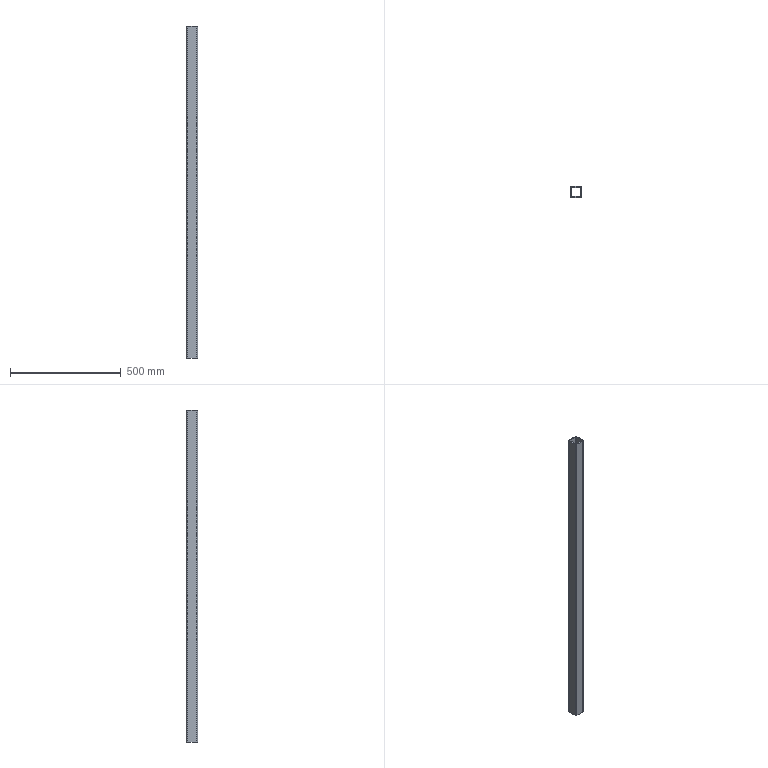Part | SolidWorks | features Extrusion 1 | 1 solid | 18 faces | box 50 x 50 x 1500 mm | volume 1304934 mm3 | plane 10 | cylinder 8 | commonest cylinder face diameters 2 x4 12 x4
STEP:
#1=CARTESIAN_POINT('',(0.,6.,1500.));
#2=VERTEX_POINT('',#1);
#3=CARTESIAN_POINT('',(6.,0.,1500.));
#4=VERTEX_POINT('',#3);
#5=CARTESIAN_POINT('',(6.,6.,1500.));
#6=DIRECTION('',(0.,0.,1.));
#7=DIRECTION('',(-1.,0.,0.));
#8=AXIS2_PLACEMENT_3D('',#5,#6,#7);
#9=CIRCLE('',#8,6.);
#10=EDGE_CURVE('',#2,#4,#9,.T.);
#11=ORIENTED_EDGE('',*,*,#10,.T.);
#12=CARTESIAN_POINT('',(44.,0.,1500.));
#13=VERTEX_POINT('',#12);
#14=CARTESIAN_POINT('',(6.,0.,1500.));
#15=DIRECTION('',(1.,0.,0.));
#16=VECTOR('',#15,1000.);
#17=LINE('',#14,#16);
#18=EDGE_CURVE('',#4,#13,#17,.T.);
#19=ORIENTED_EDGE('',*,*,#18,.T.);
#20=CARTESIAN_POINT('',(50.,6.,1500.));
#21=VERTEX_POINT('',#20);
#22=CARTESIAN_POINT('',(44.,6.,1500.));
#23=DIRECTION('',(0.,0.,1.));
#24=DIRECTION('',(1.,0.,0.));
#25=AXIS2_PLACEMENT_3D('',#22,#23,#24);
#26=CIRCLE('',#25,6.);
#27=EDGE_CURVE('',#13,#21,#26,.T.);
#28=ORIENTED_EDGE('',*,*,#27,.T.);
#29=CARTESIAN_POINT('',(50.,44.,1500.));
#30=VERTEX_POINT('',#29);
#31=CARTESIAN_POINT('',(50.,6.,1500.));
#32=DIRECTION('',(0.,1.,0.));
#33=VECTOR('',#32,1000.);
#34=LINE('',#31,#33);
#35=EDGE_CURVE('',#21,#30,#34,.T.);
#36=ORIENTED_EDGE('',*,*,#35,.T.);
#37=CARTESIAN_POINT('',(44.,50.,1500.));
#38=VERTEX_POINT('',#37);
#39=CARTESIAN_POINT('',(44.,44.,1500.));
#40=DIRECTION('',(0.,0.,1.));
#41=DIRECTION('',(-1.,0.,0.));
#42=AXIS2_PLACEMENT_3D('',#39,#40,#41);
#43=CIRCLE('',#42,6.);
#44=EDGE_CURVE('',#30,#38,#43,.T.);
#45=ORIENTED_EDGE('',*,*,#44,.T.);
#46=CARTESIAN_POINT('',(6.,50.,1500.));
#47=VERTEX_POINT('',#46);
#48=CARTESIAN_POINT('',(6.,50.,1500.));
#49=DIRECTION('',(-1.,0.,0.));
#50=VECTOR('',#49,1000.);
#51=LINE('',#48,#50);
#52=EDGE_CURVE('',#38,#47,#51,.T.);
#53=ORIENTED_EDGE('',*,*,#52,.T.);
#54=CARTESIAN_POINT('',(0.,44.,1500.));
#55=VERTEX_POINT('',#54);
#56=CARTESIAN_POINT('',(6.,44.,1500.));
#57=DIRECTION('',(0.,0.,1.));
#58=DIRECTION('',(-1.,0.,0.));
#59=AXIS2_PLACEMENT_3D('',#56,#57,#58);
#60=CIRCLE('',#59,6.);
#61=EDGE_CURVE('',#47,#55,#60,.T.);
#62=ORIENTED_EDGE('',*,*,#61,.T.);
#63=CARTESIAN_POINT('',(0.,6.,1500.));
#64=DIRECTION('',(0.,-1.,0.));
#65=VECTOR('',#64,1000.);
#66=LINE('',#63,#65);
#67=EDGE_CURVE('',#55,#2,#66,.T.);
#68=ORIENTED_EDGE('',*,*,#67,.T.);
#69=EDGE_LOOP('',(#11,#19,#28,#36,#45,#53,#62,#68));
#70=FACE_OUTER_BOUND('',#69,.T.);
#71=CARTESIAN_POINT('',(6.,45.,1500.));
#72=VERTEX_POINT('',#71);
#73=CARTESIAN_POINT('',(5.,44.,1500.));
#74=VERTEX_POINT('',#73);
#75=CARTESIAN_POINT('',(6.,44.,1500.));
#76=DIRECTION('',(0.,0.,1.));
#77=DIRECTION('',(-1.,0.,0.));
#78=AXIS2_PLACEMENT_3D('',#75,#76,#77);
#79=CIRCLE('',#78,1.);
#80=EDGE_CURVE('',#72,#74,#79,.T.);
#81=ORIENTED_EDGE('',*,*,#80,.F.);
#82=CARTESIAN_POINT('',(44.,45.,1500.));
#83=VERTEX_POINT('',#82);
#84=CARTESIAN_POINT('',(6.,45.,1500.));
#85=DIRECTION('',(-1.,0.,0.));
#86=VECTOR('',#85,1000.);
#87=LINE('',#84,#86);
#88=EDGE_CURVE('',#83,#72,#87,.T.);
#89=ORIENTED_EDGE('',*,*,#88,.F.);
#90=CARTESIAN_POINT('',(45.,44.,1500.));
#91=VERTEX_POINT('',#90);
#92=CARTESIAN_POINT('',(44.,44.,1500.));
#93=DIRECTION('',(0.,0.,1.));
#94=DIRECTION('',(-1.,0.,0.));
#95=AXIS2_PLACEMENT_3D('',#92,#93,#94);
#96=CIRCLE('',#95,1.);
#97=EDGE_CURVE('',#91,#83,#96,.T.);
#98=ORIENTED_EDGE('',*,*,#97,.F.);
#99=CARTESIAN_POINT('',(45.,6.,1500.));
#100=VERTEX_POINT('',#99);
#101=CARTESIAN_POINT('',(45.,6.,1500.));
#102=DIRECTION('',(0.,1.,0.));
#103=VECTOR('',#102,1000.);
#104=LINE('',#101,#103);
#105=EDGE_CURVE('',#100,#91,#104,.T.);
#106=ORIENTED_EDGE('',*,*,#105,.F.);
#107=CARTESIAN_POINT('',(44.,5.,1500.));
#108=VERTEX_POINT('',#107);
#109=CARTESIAN_POINT('',(44.,6.,1500.));
#110=DIRECTION('',(0.,0.,1.));
#111=DIRECTION('',(1.,0.,0.));
#112=AXIS2_PLACEMENT_3D('',#109,#110,#111);
#113=CIRCLE('',#112,1.);
#114=EDGE_CURVE('',#108,#100,#113,.T.);
#115=ORIENTED_EDGE('',*,*,#114,.F.);
#116=CARTESIAN_POINT('',(6.,5.,1500.));
#117=VERTEX_POINT('',#116);
#118=CARTESIAN_POINT('',(6.,5.,1500.));
#119=DIRECTION('',(1.,0.,0.));
#120=VECTOR('',#119,1000.);
#121=LINE('',#118,#120);
#122=EDGE_CURVE('',#117,#108,#121,.T.);
#123=ORIENTED_EDGE('',*,*,#122,.F.);
#124=CARTESIAN_POINT('',(5.,6.,1500.));
#125=VERTEX_POINT('',#124);
#126=CARTESIAN_POINT('',(6.,6.,1500.));
#127=DIRECTION('',(0.,0.,1.));
#128=DIRECTION('',(-1.,0.,0.));
#129=AXIS2_PLACEMENT_3D('',#126,#127,#128);
#130=CIRCLE('',#129,1.);
#131=EDGE_CURVE('',#125,#117,#130,.T.);
#132=ORIENTED_EDGE('',*,*,#131,.F.);
#133=CARTESIAN_POINT('',(5.,6.,1500.));
#134=DIRECTION('',(0.,-1.,0.));
#135=VECTOR('',#134,1000.);
#136=LINE('',#133,#135);
#137=EDGE_CURVE('',#74,#125,#136,.T.);
#138=ORIENTED_EDGE('',*,*,#137,.F.);
#139=EDGE_LOOP('',(#81,#89,#98,#106,#115,#123,#132,#138));
#140=FACE_BOUND('',#139,.T.);
#141=CARTESIAN_POINT('',(6.,6.,1500.));
#142=DIRECTION('',(0.,0.,-1.));
#143=DIRECTION('',(-1.,0.,0.));
#144=AXIS2_PLACEMENT_3D('',#141,#142,#143);
#145=PLANE('',#144);
#146=ADVANCED_FACE('',(#70,#140),#145,.F.);
#147=CARTESIAN_POINT('',(0.,6.,0.));
#148=VERTEX_POINT('',#147);
#149=CARTESIAN_POINT('',(6.,0.,0.));
#150=VERTEX_POINT('',#149);
#151=CARTESIAN_POINT('',(6.,6.,0.));
#152=DIRECTION('',(0.,0.,1.));
#153=DIRECTION('',(-1.,0.,0.));
#154=AXIS2_PLACEMENT_3D('',#151,#152,#153);
#155=CIRCLE('',#154,6.);
#156=EDGE_CURVE('',#148,#150,#155,.T.);
#157=ORIENTED_EDGE('',*,*,#156,.F.);
#158=CARTESIAN_POINT('',(0.,44.,0.));
#159=VERTEX_POINT('',#158);
#160=CARTESIAN_POINT('',(0.,6.,0.));
#161=DIRECTION('',(0.,-1.,0.));
#162=VECTOR('',#161,1000.);
#163=LINE('',#160,#162);
#164=EDGE_CURVE('',#159,#148,#163,.T.);
#165=ORIENTED_EDGE('',*,*,#164,.F.);
#166=CARTESIAN_POINT('',(6.,50.,0.));
#167=VERTEX_POINT('',#166);
#168=CARTESIAN_POINT('',(6.,44.,0.));
#169=DIRECTION('',(0.,0.,1.));
#170=DIRECTION('',(-1.,0.,0.));
#171=AXIS2_PLACEMENT_3D('',#168,#169,#170);
#172=CIRCLE('',#171,6.);
#173=EDGE_CURVE('',#167,#159,#172,.T.);
#174=ORIENTED_EDGE('',*,*,#173,.F.);
#175=CARTESIAN_POINT('',(44.,50.,0.));
#176=VERTEX_POINT('',#175);
#177=CARTESIAN_POINT('',(6.,50.,0.));
#178=DIRECTION('',(-1.,0.,0.));
#179=VECTOR('',#178,1000.);
#180=LINE('',#177,#179);
#181=EDGE_CURVE('',#176,#167,#180,.T.);
#182=ORIENTED_EDGE('',*,*,#181,.F.);
#183=CARTESIAN_POINT('',(50.,44.,0.));
#184=VERTEX_POINT('',#183);
#185=CARTESIAN_POINT('',(44.,44.,0.));
#186=DIRECTION('',(0.,0.,1.));
#187=DIRECTION('',(-1.,0.,0.));
#188=AXIS2_PLACEMENT_3D('',#185,#186,#187);
#189=CIRCLE('',#188,6.);
#190=EDGE_CURVE('',#184,#176,#189,.T.);
#191=ORIENTED_EDGE('',*,*,#190,.F.);
#192=CARTESIAN_POINT('',(50.,6.,0.));
#193=VERTEX_POINT('',#192);
#194=CARTESIAN_POINT('',(50.,6.,0.));
#195=DIRECTION('',(0.,1.,0.));
#196=VECTOR('',#195,1000.);
#197=LINE('',#194,#196);
#198=EDGE_CURVE('',#193,#184,#197,.T.);
#199=ORIENTED_EDGE('',*,*,#198,.F.);
#200=CARTESIAN_POINT('',(44.,0.,0.));
#201=VERTEX_POINT('',#200);
#202=CARTESIAN_POINT('',(44.,6.,0.));
#203=DIRECTION('',(0.,0.,1.));
#204=DIRECTION('',(1.,0.,0.));
#205=AXIS2_PLACEMENT_3D('',#202,#203,#204);
#206=CIRCLE('',#205,6.);
#207=EDGE_CURVE('',#201,#193,#206,.T.);
#208=ORIENTED_EDGE('',*,*,#207,.F.);
#209=CARTESIAN_POINT('',(6.,0.,0.));
#210=DIRECTION('',(1.,0.,0.));
#211=VECTOR('',#210,1000.);
#212=LINE('',#209,#211);
#213=EDGE_CURVE('',#150,#201,#212,.T.);
#214=ORIENTED_EDGE('',*,*,#213,.F.);
#215=EDGE_LOOP('',(#157,#165,#174,#182,#191,#199,#208,#214));
#216=FACE_OUTER_BOUND('',#215,.T.);
#217=CARTESIAN_POINT('',(44.,45.,0.));
#218=VERTEX_POINT('',#217);
#219=CARTESIAN_POINT('',(6.,45.,0.));
#220=VERTEX_POINT('',#219);
#221=CARTESIAN_POINT('',(6.,45.,0.));
#222=DIRECTION('',(-1.,0.,0.));
#223=VECTOR('',#222,1000.);
#224=LINE('',#221,#223);
#225=EDGE_CURVE('',#218,#220,#224,.T.);
#226=ORIENTED_EDGE('',*,*,#225,.T.);
#227=CARTESIAN_POINT('',(5.,44.,0.));
#228=VERTEX_POINT('',#227);
#229=CARTESIAN_POINT('',(6.,44.,0.));
#230=DIRECTION('',(0.,0.,1.));
#231=DIRECTION('',(-1.,0.,0.));
#232=AXIS2_PLACEMENT_3D('',#229,#230,#231);
#233=CIRCLE('',#232,1.);
#234=EDGE_CURVE('',#220,#228,#233,.T.);
#235=ORIENTED_EDGE('',*,*,#234,.T.);
#236=CARTESIAN_POINT('',(5.,6.,0.));
#237=VERTEX_POINT('',#236);
#238=CARTESIAN_POINT('',(5.,6.,0.));
#239=DIRECTION('',(0.,-1.,0.));
#240=VECTOR('',#239,1000.);
#241=LINE('',#238,#240);
#242=EDGE_CURVE('',#228,#237,#241,.T.);
#243=ORIENTED_EDGE('',*,*,#242,.T.);
#244=CARTESIAN_POINT('',(6.,5.,0.));
#245=VERTEX_POINT('',#244);
#246=CARTESIAN_POINT('',(6.,6.,0.));
#247=DIRECTION('',(0.,0.,1.));
#248=DIRECTION('',(-1.,0.,0.));
#249=AXIS2_PLACEMENT_3D('',#246,#247,#248);
#250=CIRCLE('',#249,1.);
#251=EDGE_CURVE('',#237,#245,#250,.T.);
#252=ORIENTED_EDGE('',*,*,#251,.T.);
#253=CARTESIAN_POINT('',(44.,5.,0.));
#254=VERTEX_POINT('',#253);
#255=CARTESIAN_POINT('',(6.,5.,0.));
#256=DIRECTION('',(1.,0.,0.));
#257=VECTOR('',#256,1000.);
#258=LINE('',#255,#257);
#259=EDGE_CURVE('',#245,#254,#258,.T.);
#260=ORIENTED_EDGE('',*,*,#259,.T.);
#261=CARTESIAN_POINT('',(45.,6.,0.));
#262=VERTEX_POINT('',#261);
#263=CARTESIAN_POINT('',(44.,6.,0.));
#264=DIRECTION('',(0.,0.,1.));
#265=DIRECTION('',(1.,0.,0.));
#266=AXIS2_PLACEMENT_3D('',#263,#264,#265);
#267=CIRCLE('',#266,1.);
#268=EDGE_CURVE('',#254,#262,#267,.T.);
#269=ORIENTED_EDGE('',*,*,#268,.T.);
#270=CARTESIAN_POINT('',(45.,44.,0.));
#271=VERTEX_POINT('',#270);
#272=CARTESIAN_POINT('',(45.,6.,0.));
#273=DIRECTION('',(0.,1.,0.));
#274=VECTOR('',#273,1000.);
#275=LINE('',#272,#274);
#276=EDGE_CURVE('',#262,#271,#275,.T.);
#277=ORIENTED_EDGE('',*,*,#276,.T.);
#278=CARTESIAN_POINT('',(44.,44.,0.));
#279=DIRECTION('',(0.,0.,1.));
#280=DIRECTION('',(-1.,0.,0.));
#281=AXIS2_PLACEMENT_3D('',#278,#279,#280);
#282=CIRCLE('',#281,1.);
#283=EDGE_CURVE('',#271,#218,#282,.T.);
#284=ORIENTED_EDGE('',*,*,#283,.T.);
#285=EDGE_LOOP('',(#226,#235,#243,#252,#260,#269,#277,#284));
#286=FACE_BOUND('',#285,.T.);
#287=CARTESIAN_POINT('',(6.,6.,0.));
#288=DIRECTION('',(0.,0.,-1.));
#289=DIRECTION('',(-1.,0.,0.));
#290=AXIS2_PLACEMENT_3D('',#287,#288,#289);
#291=PLANE('',#290);
#292=ADVANCED_FACE('',(#216,#286),#291,.T.);
#293=ORIENTED_EDGE('',*,*,#156,.T.);
#294=CARTESIAN_POINT('',(6.,0.,1500.));
#295=DIRECTION('',(0.,0.,-1.));
#296=VECTOR('',#295,1000.);
#297=LINE('',#294,#296);
#298=EDGE_CURVE('',#4,#150,#297,.T.);
#299=ORIENTED_EDGE('',*,*,#298,.F.);
#300=ORIENTED_EDGE('',*,*,#10,.F.);
#301=CARTESIAN_POINT('',(0.,6.,1500.));
#302=DIRECTION('',(0.,0.,-1.));
#303=VECTOR('',#302,1000.);
#304=LINE('',#301,#303);
#305=EDGE_CURVE('',#2,#148,#304,.T.);
#306=ORIENTED_EDGE('',*,*,#305,.T.);
#307=EDGE_LOOP('',(#293,#299,#300,#306));
#308=FACE_OUTER_BOUND('',#307,.T.);
#309=CARTESIAN_POINT('',(6.,6.,1500.));
#310=DIRECTION('',(0.,0.,-1.));
#311=DIRECTION('',(-1.,0.,0.));
#312=AXIS2_PLACEMENT_3D('',#309,#310,#311);
#313=CYLINDRICAL_SURFACE('',#312,6.);
#314=ADVANCED_FACE('',(#308),#313,.T.);
#315=ORIENTED_EDGE('',*,*,#213,.T.);
#316=CARTESIAN_POINT('',(44.,0.,1500.));
#317=DIRECTION('',(0.,0.,-1.));
#318=VECTOR('',#317,1000.);
#319=LINE('',#316,#318);
#320=EDGE_CURVE('',#13,#201,#319,.T.);
#321=ORIENTED_EDGE('',*,*,#320,.F.);
#322=ORIENTED_EDGE('',*,*,#18,.F.);
#323=ORIENTED_EDGE('',*,*,#298,.T.);
#324=EDGE_LOOP('',(#315,#321,#322,#323));
#325=FACE_OUTER_BOUND('',#324,.T.);
#326=CARTESIAN_POINT('',(6.,0.,1500.));
#327=DIRECTION('',(0.,1.,0.));
#328=DIRECTION('',(0.,0.,1.));
#329=AXIS2_PLACEMENT_3D('',#326,#327,#328);
#330=PLANE('',#329);
#331=ADVANCED_FACE('',(#325),#330,.F.);
#332=ORIENTED_EDGE('',*,*,#207,.T.);
#333=CARTESIAN_POINT('',(50.,6.,1500.));
#334=DIRECTION('',(0.,0.,-1.));
#335=VECTOR('',#334,1000.);
#336=LINE('',#333,#335);
#337=EDGE_CURVE('',#21,#193,#336,.T.);
#338=ORIENTED_EDGE('',*,*,#337,.F.);
#339=ORIENTED_EDGE('',*,*,#27,.F.);
#340=ORIENTED_EDGE('',*,*,#320,.T.);
#341=EDGE_LOOP('',(#332,#338,#339,#340));
#342=FACE_OUTER_BOUND('',#341,.T.);
#343=CARTESIAN_POINT('',(44.,6.,1500.));
#344=DIRECTION('',(0.,0.,-1.));
#345=DIRECTION('',(-1.,0.,0.));
#346=AXIS2_PLACEMENT_3D('',#343,#344,#345);
#347=CYLINDRICAL_SURFACE('',#346,6.);
#348=ADVANCED_FACE('',(#342),#347,.T.);
#349=ORIENTED_EDGE('',*,*,#198,.T.);
#350=CARTESIAN_POINT('',(50.,44.,1500.));
#351=DIRECTION('',(0.,0.,-1.));
#352=VECTOR('',#351,1000.);
#353=LINE('',#350,#352);
#354=EDGE_CURVE('',#30,#184,#353,.T.);
#355=ORIENTED_EDGE('',*,*,#354,.F.);
#356=ORIENTED_EDGE('',*,*,#35,.F.);
#357=ORIENTED_EDGE('',*,*,#337,.T.);
#358=EDGE_LOOP('',(#349,#355,#356,#357));
#359=FACE_OUTER_BOUND('',#358,.T.);
#360=CARTESIAN_POINT('',(50.,6.,1500.));
#361=DIRECTION('',(-1.,0.,0.));
#362=DIRECTION('',(0.,0.,1.));
#363=AXIS2_PLACEMENT_3D('',#360,#361,#362);
#364=PLANE('',#363);
#365=ADVANCED_FACE('',(#359),#364,.F.);
#366=ORIENTED_EDGE('',*,*,#190,.T.);
#367=CARTESIAN_POINT('',(44.,50.,1500.));
#368=DIRECTION('',(0.,0.,-1.));
#369=VECTOR('',#368,1000.);
#370=LINE('',#367,#369);
#371=EDGE_CURVE('',#38,#176,#370,.T.);
#372=ORIENTED_EDGE('',*,*,#371,.F.);
#373=ORIENTED_EDGE('',*,*,#44,.F.);
#374=ORIENTED_EDGE('',*,*,#354,.T.);
#375=EDGE_LOOP('',(#366,#372,#373,#374));
#376=FACE_OUTER_BOUND('',#375,.T.);
#377=CARTESIAN_POINT('',(44.,44.,1500.));
#378=DIRECTION('',(0.,0.,-1.));
#379=DIRECTION('',(-1.,0.,0.));
#380=AXIS2_PLACEMENT_3D('',#377,#378,#379);
#381=CYLINDRICAL_SURFACE('',#380,6.);
#382=ADVANCED_FACE('',(#376),#381,.T.);
#383=ORIENTED_EDGE('',*,*,#181,.T.);
#384=CARTESIAN_POINT('',(6.,50.,1500.));
#385=DIRECTION('',(0.,0.,-1.));
#386=VECTOR('',#385,1000.);
#387=LINE('',#384,#386);
#388=EDGE_CURVE('',#47,#167,#387,.T.);
#389=ORIENTED_EDGE('',*,*,#388,.F.);
#390=ORIENTED_EDGE('',*,*,#52,.F.);
#391=ORIENTED_EDGE('',*,*,#371,.T.);
#392=EDGE_LOOP('',(#383,#389,#390,#391));
#393=FACE_OUTER_BOUND('',#392,.T.);
#394=CARTESIAN_POINT('',(6.,50.,1500.));
#395=DIRECTION('',(0.,-1.,0.));
#396=DIRECTION('',(0.,0.,-1.));
#397=AXIS2_PLACEMENT_3D('',#394,#395,#396);
#398=PLANE('',#397);
#399=ADVANCED_FACE('',(#393),#398,.F.);
#400=ORIENTED_EDGE('',*,*,#173,.T.);
#401=CARTESIAN_POINT('',(0.,44.,1500.));
#402=DIRECTION('',(0.,0.,-1.));
#403=VECTOR('',#402,1000.);
#404=LINE('',#401,#403);
#405=EDGE_CURVE('',#55,#159,#404,.T.);
#406=ORIENTED_EDGE('',*,*,#405,.F.);
#407=ORIENTED_EDGE('',*,*,#61,.F.);
#408=ORIENTED_EDGE('',*,*,#388,.T.);
#409=EDGE_LOOP('',(#400,#406,#407,#408));
#410=FACE_OUTER_BOUND('',#409,.T.);
#411=CARTESIAN_POINT('',(6.,44.,1500.));
#412=DIRECTION('',(0.,0.,-1.));
#413=DIRECTION('',(-1.,0.,0.));
#414=AXIS2_PLACEMENT_3D('',#411,#412,#413);
#415=CYLINDRICAL_SURFACE('',#414,6.);
#416=ADVANCED_FACE('',(#410),#415,.T.);
#417=ORIENTED_EDGE('',*,*,#164,.T.);
#418=ORIENTED_EDGE('',*,*,#305,.F.);
#419=ORIENTED_EDGE('',*,*,#67,.F.);
#420=ORIENTED_EDGE('',*,*,#405,.T.);
#421=EDGE_LOOP('',(#417,#418,#419,#420));
#422=FACE_OUTER_BOUND('',#421,.T.);
#423=CARTESIAN_POINT('',(0.,6.,1500.));
#424=DIRECTION('',(1.,0.,0.));
#425=DIRECTION('',(0.,0.,-1.));
#426=AXIS2_PLACEMENT_3D('',#423,#424,#425);
#427=PLANE('',#426);
#428=ADVANCED_FACE('',(#422),#427,.F.);
#429=ORIENTED_EDGE('',*,*,#234,.F.);
#430=CARTESIAN_POINT('',(6.,45.,1500.));
#431=DIRECTION('',(0.,0.,-1.));
#432=VECTOR('',#431,1000.);
#433=LINE('',#430,#432);
#434=EDGE_CURVE('',#72,#220,#433,.T.);
#435=ORIENTED_EDGE('',*,*,#434,.F.);
#436=ORIENTED_EDGE('',*,*,#80,.T.);
#437=CARTESIAN_POINT('',(5.,44.,1500.));
#438=DIRECTION('',(0.,0.,-1.));
#439=VECTOR('',#438,1000.);
#440=LINE('',#437,#439);
#441=EDGE_CURVE('',#74,#228,#440,.T.);
#442=ORIENTED_EDGE('',*,*,#441,.T.);
#443=EDGE_LOOP('',(#429,#435,#436,#442));
#444=FACE_OUTER_BOUND('',#443,.T.);
#445=CARTESIAN_POINT('',(6.,44.,1500.));
#446=DIRECTION('',(0.,0.,-1.));
#447=DIRECTION('',(-1.,0.,0.));
#448=AXIS2_PLACEMENT_3D('',#445,#446,#447);
#449=CYLINDRICAL_SURFACE('',#448,1.);
#450=ADVANCED_FACE('',(#444),#449,.F.);
#451=ORIENTED_EDGE('',*,*,#242,.F.);
#452=ORIENTED_EDGE('',*,*,#441,.F.);
#453=ORIENTED_EDGE('',*,*,#137,.T.);
#454=CARTESIAN_POINT('',(5.,6.,1500.));
#455=DIRECTION('',(0.,0.,-1.));
#456=VECTOR('',#455,1000.);
#457=LINE('',#454,#456);
#458=EDGE_CURVE('',#125,#237,#457,.T.);
#459=ORIENTED_EDGE('',*,*,#458,.T.);
#460=EDGE_LOOP('',(#451,#452,#453,#459));
#461=FACE_OUTER_BOUND('',#460,.T.);
#462=CARTESIAN_POINT('',(5.,6.,1500.));
#463=DIRECTION('',(1.,0.,0.));
#464=DIRECTION('',(0.,1.,0.));
#465=AXIS2_PLACEMENT_3D('',#462,#463,#464);
#466=PLANE('',#465);
#467=ADVANCED_FACE('',(#461),#466,.T.);
#468=ORIENTED_EDGE('',*,*,#251,.F.);
#469=ORIENTED_EDGE('',*,*,#458,.F.);
#470=ORIENTED_EDGE('',*,*,#131,.T.);
#471=CARTESIAN_POINT('',(6.,5.,1500.));
#472=DIRECTION('',(0.,0.,-1.));
#473=VECTOR('',#472,1000.);
#474=LINE('',#471,#473);
#475=EDGE_CURVE('',#117,#245,#474,.T.);
#476=ORIENTED_EDGE('',*,*,#475,.T.);
#477=EDGE_LOOP('',(#468,#469,#470,#476));
#478=FACE_OUTER_BOUND('',#477,.T.);
#479=CARTESIAN_POINT('',(6.,6.,1500.));
#480=DIRECTION('',(0.,0.,-1.));
#481=DIRECTION('',(-1.,0.,0.));
#482=AXIS2_PLACEMENT_3D('',#479,#480,#481);
#483=CYLINDRICAL_SURFACE('',#482,1.);
#484=ADVANCED_FACE('',(#478),#483,.F.);
#485=ORIENTED_EDGE('',*,*,#259,.F.);
#486=ORIENTED_EDGE('',*,*,#475,.F.);
#487=ORIENTED_EDGE('',*,*,#122,.T.);
#488=CARTESIAN_POINT('',(44.,5.,1500.));
#489=DIRECTION('',(0.,0.,-1.));
#490=VECTOR('',#489,1000.);
#491=LINE('',#488,#490);
#492=EDGE_CURVE('',#108,#254,#491,.T.);
#493=ORIENTED_EDGE('',*,*,#492,.T.);
#494=EDGE_LOOP('',(#485,#486,#487,#493));
#495=FACE_OUTER_BOUND('',#494,.T.);
#496=CARTESIAN_POINT('',(6.,5.,1500.));
#497=DIRECTION('',(0.,1.,0.));
#498=DIRECTION('',(-1.,0.,0.));
#499=AXIS2_PLACEMENT_3D('',#496,#497,#498);
#500=PLANE('',#499);
#501=ADVANCED_FACE('',(#495),#500,.T.);
#502=ORIENTED_EDGE('',*,*,#268,.F.);
#503=ORIENTED_EDGE('',*,*,#492,.F.);
#504=ORIENTED_EDGE('',*,*,#114,.T.);
#505=CARTESIAN_POINT('',(45.,6.,1500.));
#506=DIRECTION('',(0.,0.,-1.));
#507=VECTOR('',#506,1000.);
#508=LINE('',#505,#507);
#509=EDGE_CURVE('',#100,#262,#508,.T.);
#510=ORIENTED_EDGE('',*,*,#509,.T.);
#511=EDGE_LOOP('',(#502,#503,#504,#510));
#512=FACE_OUTER_BOUND('',#511,.T.);
#513=CARTESIAN_POINT('',(44.,6.,1500.));
#514=DIRECTION('',(0.,0.,-1.));
#515=DIRECTION('',(-1.,0.,0.));
#516=AXIS2_PLACEMENT_3D('',#513,#514,#515);
#517=CYLINDRICAL_SURFACE('',#516,1.);
#518=ADVANCED_FACE('',(#512),#517,.F.);
#519=ORIENTED_EDGE('',*,*,#276,.F.);
#520=ORIENTED_EDGE('',*,*,#509,.F.);
#521=ORIENTED_EDGE('',*,*,#105,.T.);
#522=CARTESIAN_POINT('',(45.,44.,1500.));
#523=DIRECTION('',(0.,0.,-1.));
#524=VECTOR('',#523,1000.);
#525=LINE('',#522,#524);
#526=EDGE_CURVE('',#91,#271,#525,.T.);
#527=ORIENTED_EDGE('',*,*,#526,.T.);
#528=EDGE_LOOP('',(#519,#520,#521,#527));
#529=FACE_OUTER_BOUND('',#528,.T.);
#530=CARTESIAN_POINT('',(45.,6.,1500.));
#531=DIRECTION('',(-1.,0.,0.));
#532=DIRECTION('',(0.,0.,1.));
#533=AXIS2_PLACEMENT_3D('',#530,#531,#532);
#534=PLANE('',#533);
#535=ADVANCED_FACE('',(#529),#534,.T.);
#536=ORIENTED_EDGE('',*,*,#283,.F.);
#537=ORIENTED_EDGE('',*,*,#526,.F.);
#538=ORIENTED_EDGE('',*,*,#97,.T.);
#539=CARTESIAN_POINT('',(44.,45.,1500.));
#540=DIRECTION('',(0.,0.,-1.));
#541=VECTOR('',#540,1000.);
#542=LINE('',#539,#541);
#543=EDGE_CURVE('',#83,#218,#542,.T.);
#544=ORIENTED_EDGE('',*,*,#543,.T.);
#545=EDGE_LOOP('',(#536,#537,#538,#544));
#546=FACE_OUTER_BOUND('',#545,.T.);
#547=CARTESIAN_POINT('',(44.,44.,1500.));
#548=DIRECTION('',(0.,0.,-1.));
#549=DIRECTION('',(-1.,0.,0.));
#550=AXIS2_PLACEMENT_3D('',#547,#548,#549);
#551=CYLINDRICAL_SURFACE('',#550,1.);
#552=ADVANCED_FACE('',(#546),#551,.F.);
#553=ORIENTED_EDGE('',*,*,#225,.F.);
#554=ORIENTED_EDGE('',*,*,#543,.F.);
#555=ORIENTED_EDGE('',*,*,#88,.T.);
#556=ORIENTED_EDGE('',*,*,#434,.T.);
#557=EDGE_LOOP('',(#553,#554,#555,#556));
#558=FACE_OUTER_BOUND('',#557,.T.);
#559=CARTESIAN_POINT('',(6.,45.,1500.));
#560=DIRECTION('',(0.,-1.,0.));
#561=DIRECTION('',(0.,0.,-1.));
#562=AXIS2_PLACEMENT_3D('',#559,#560,#561);
#563=PLANE('',#562);
#564=ADVANCED_FACE('',(#558),#563,.T.);
#565=CLOSED_SHELL('',(#146,#292,#314,#331,#348,#365,#382,#399,#416,#428,#450,#467,#484,#501,#518,#535,#552,#564));
#566=MANIFOLD_SOLID_BREP('',#565);
#567=CARTESIAN_POINT('',(0.,0.,0.));
#568=DIRECTION('',(0.,0.,1.));
#569=DIRECTION('',(1.,0.,0.));
#570=AXIS2_PLACEMENT_3D('',#567,#568,#569);
#571=(LENGTH_UNIT()NAMED_UNIT(*)SI_UNIT(.MILLI.,.METRE.));
#572=UNCERTAINTY_MEASURE_WITH_UNIT(LENGTH_MEASURE(0.00001),#571,'','');
#573=(NAMED_UNIT(*)PLANE_ANGLE_UNIT()SI_UNIT($,.RADIAN.));
#574=(NAMED_UNIT(*)SI_UNIT($,.STERADIAN.)SOLID_ANGLE_UNIT());
#575=(GEOMETRIC_REPRESENTATION_CONTEXT(3)GLOBAL_UNCERTAINTY_ASSIGNED_CONTEXT((#572))GLOBAL_UNIT_ASSIGNED_CONTEXT((#571,#573,#574))REPRESENTATION_CONTEXT('',''));
#576=ADVANCED_BREP_SHAPE_REPRESENTATION('',(#566,#570),#575);